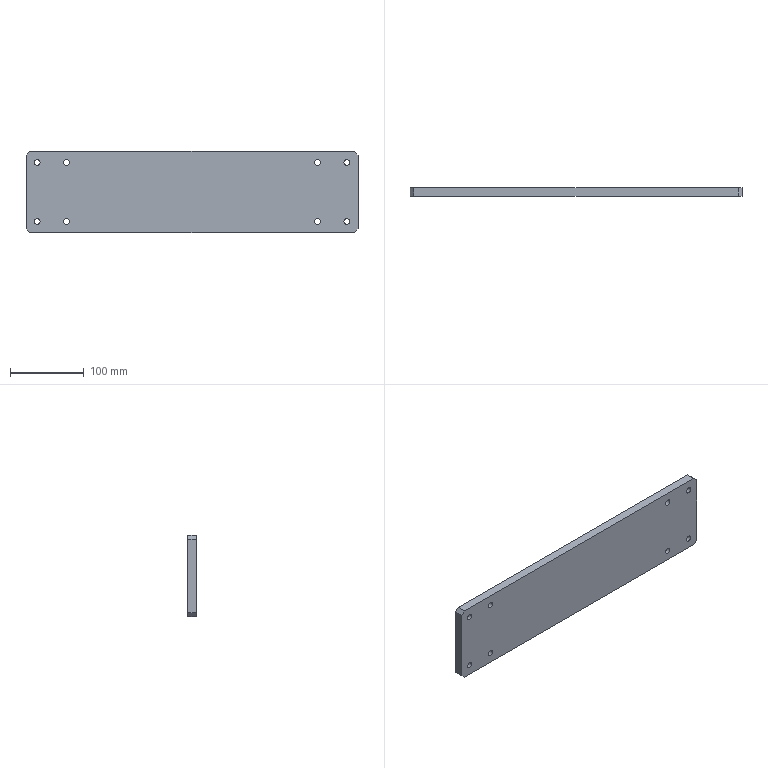Part | STEP file | ATTACH.PLATE.stp | 1 solid | 26 faces | box 450 x 12 x 110 mm | volume 588575 mm3 | spline 15 | cylinder 8 | plane 3 | commonest cylinder face diameters 8 x8